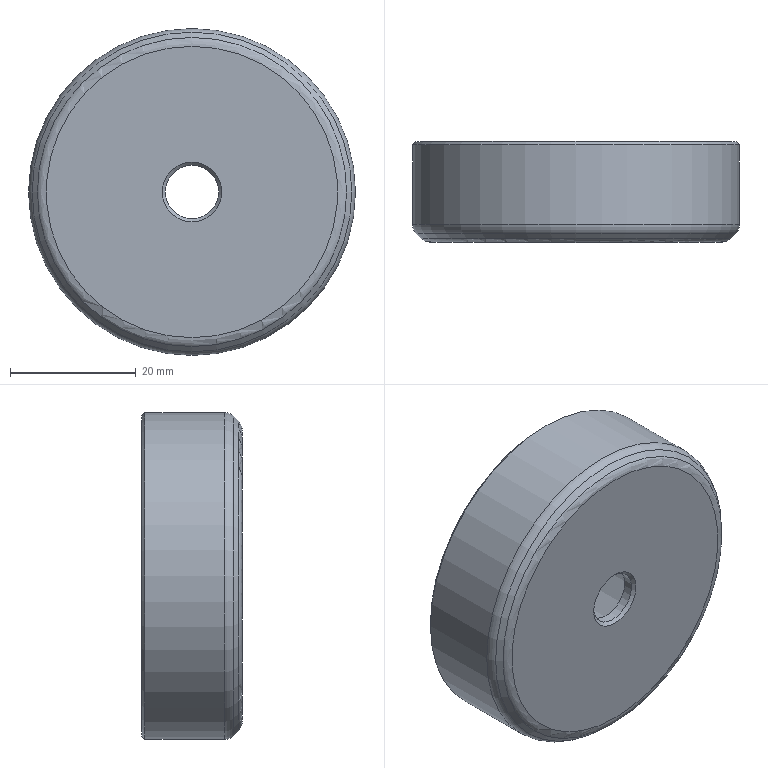Part | STEP file | PN_0026_default | 1 solid | 21 faces | box 52 x 16 x 52 mm | volume 11242 mm3 | torus 8 | cylinder 5 | plane 5 | cone 3 | commonest cylinder face diameters 8.5 x1 33 x1 37 x1 48 x1 52 x1
STEP:
#1=CARTESIAN_POINT('',(0.,0.,0.));
#2=DIRECTION('',(0.,0.,1.));
#3=DIRECTION('',(1.,0.,0.));
#4=AXIS2_PLACEMENT_3D('',#1,#2,#3);
#5=CARTESIAN_POINT('',(0.,0.5,4.25));
#6=VERTEX_POINT('',#5);
#7=CARTESIAN_POINT('',(0.,0.5,0.));
#8=DIRECTION('',(0.,-1.,0.));
#9=DIRECTION('',(0.,0.,1.));
#10=AXIS2_PLACEMENT_3D('',#7,#8,#9);
#11=CIRCLE('',#10,4.25);
#12=CARTESIAN_POINT('',(0.,49.95,0.));
#13=DIRECTION('',(0.,1.,0.));
#14=DIRECTION('',(0.,0.,1.));
#15=AXIS2_PLACEMENT_3D('',#12,#13,#14);
#16=CYLINDRICAL_SURFACE('',#15,4.25);
#17=CARTESIAN_POINT('',(6.283,-49.45));
#18=DIRECTION('',(-1.,0.));
#19=VECTOR('',#18,1.);
#20=LINE('',#17,#19);
#21=(GEOMETRIC_REPRESENTATION_CONTEXT(2)PARAMETRIC_REPRESENTATION_CONTEXT()REPRESENTATION_CONTEXT('',''));
#22=DEFINITIONAL_REPRESENTATION('',(#20),#21);
#23=PCURVE('',#16,#22);
#24=CARTESIAN_POINT('',(0.,0.,0.));
#25=DIRECTION('',(0.,-1.,0.));
#26=DIRECTION('',(0.,0.,-1.));
#27=AXIS2_PLACEMENT_3D('',#24,#25,#26);
#28=CONICAL_SURFACE('',#27,4.75,0.7854);
#29=CARTESIAN_POINT('',(3.142,-0.5));
#30=DIRECTION('',(1.,0.));
#31=VECTOR('',#30,1.);
#32=LINE('',#29,#31);
#33=(GEOMETRIC_REPRESENTATION_CONTEXT(2)PARAMETRIC_REPRESENTATION_CONTEXT()REPRESENTATION_CONTEXT('',''));
#34=DEFINITIONAL_REPRESENTATION('',(#32),#33);
#35=PCURVE('',#28,#34);
#36=SURFACE_CURVE('',#11,(#23,#35),.PCURVE_S1.);
#37=EDGE_CURVE('',#6,#6,#36,.T.);
#38=ORIENTED_EDGE('',*,*,#37,.F.);
#39=CARTESIAN_POINT('',(0.,2.,4.25));
#40=VERTEX_POINT('',#39);
#41=CARTESIAN_POINT('',(0.,0.5,4.25));
#42=CARTESIAN_POINT('',(0.,2.,4.25));
#43=B_SPLINE_CURVE_WITH_KNOTS('',1,(#41,#42),.UNSPECIFIED.,.F.,.F.,(2,2),(-49.45,-47.95),.PIECEWISE_BEZIER_KNOTS.);
#44=CARTESIAN_POINT('',(6.283,0.));
#45=DIRECTION('',(0.,1.));
#46=VECTOR('',#45,1.);
#47=LINE('',#44,#46);
#48=(GEOMETRIC_REPRESENTATION_CONTEXT(2)PARAMETRIC_REPRESENTATION_CONTEXT()REPRESENTATION_CONTEXT('',''));
#49=DEFINITIONAL_REPRESENTATION('',(#47),#48);
#50=PCURVE('',#16,#49);
#51=CARTESIAN_POINT('',(0.,0.));
#52=DIRECTION('',(0.,1.));
#53=VECTOR('',#52,1.);
#54=LINE('',#51,#53);
#55=(GEOMETRIC_REPRESENTATION_CONTEXT(2)PARAMETRIC_REPRESENTATION_CONTEXT()REPRESENTATION_CONTEXT('',''));
#56=DEFINITIONAL_REPRESENTATION('',(#54),#55);
#57=PCURVE('',#16,#56);
#58=SEAM_CURVE('',#43,(#50,#57),.PCURVE_S1.);
#59=EDGE_CURVE('',#6,#40,#58,.T.);
#60=ORIENTED_EDGE('',*,*,#59,.T.);
#61=CARTESIAN_POINT('',(0.,2.,0.));
#62=DIRECTION('',(0.,1.,0.));
#63=DIRECTION('',(0.,0.,1.));
#64=AXIS2_PLACEMENT_3D('',#61,#62,#63);
#65=CIRCLE('',#64,4.25);
#66=CARTESIAN_POINT('',(0.,-47.95));
#67=DIRECTION('',(1.,0.));
#68=VECTOR('',#67,1.);
#69=LINE('',#66,#68);
#70=(GEOMETRIC_REPRESENTATION_CONTEXT(2)PARAMETRIC_REPRESENTATION_CONTEXT()REPRESENTATION_CONTEXT('',''));
#71=DEFINITIONAL_REPRESENTATION('',(#69),#70);
#72=PCURVE('',#16,#71);
#73=CARTESIAN_POINT('',(16.,2.,0.));
#74=DIRECTION('',(0.,-1.,0.));
#75=DIRECTION('',(0.,0.,-1.));
#76=AXIS2_PLACEMENT_3D('',#73,#74,#75);
#77=PLANE('',#76);
#78=CARTESIAN_POINT('',(-4.25,-16.));
#79=CARTESIAN_POINT('',(-4.25,-8.639));
#80=CARTESIAN_POINT('',(2.125,-12.319));
#81=CARTESIAN_POINT('',(8.5,-16.));
#82=CARTESIAN_POINT('',(2.125,-19.681));
#83=CARTESIAN_POINT('',(-4.25,-23.361));
#84=CARTESIAN_POINT('',(-4.25,-16.));
#85=(BOUNDED_CURVE()B_SPLINE_CURVE(2,(#78,#79,#80,#81,#82,#83,#84),.UNSPECIFIED.,.T.,.F.)B_SPLINE_CURVE_WITH_KNOTS((1,2,2,2,2,1),(-2.094,0.,2.094,4.189,6.283,8.378),.UNSPECIFIED.)CURVE()GEOMETRIC_REPRESENTATION_ITEM()RATIONAL_B_SPLINE_CURVE((1.,0.5,1.,0.5,1.,0.5,1.))REPRESENTATION_ITEM(''));
#86=(GEOMETRIC_REPRESENTATION_CONTEXT(2)PARAMETRIC_REPRESENTATION_CONTEXT()REPRESENTATION_CONTEXT('',''));
#87=DEFINITIONAL_REPRESENTATION('',(#85),#86);
#88=PCURVE('',#77,#87);
#89=SURFACE_CURVE('',#65,(#72,#88),.PCURVE_S1.);
#90=EDGE_CURVE('',#40,#40,#89,.T.);
#91=ORIENTED_EDGE('',*,*,#90,.F.);
#92=ORIENTED_EDGE('',*,*,#59,.F.);
#93=EDGE_LOOP('',(#38,#60,#91,#92));
#94=FACE_BOUND('',#93,.F.);
#95=ADVANCED_FACE('',(#94),#16,.F.);
#96=CARTESIAN_POINT('',(0.,0.,4.75));
#97=VERTEX_POINT('',#96);
#98=CARTESIAN_POINT('',(0.,0.,0.));
#99=DIRECTION('',(0.,1.,0.));
#100=DIRECTION('',(0.,0.,1.));
#101=AXIS2_PLACEMENT_3D('',#98,#99,#100);
#102=CIRCLE('',#101,4.75);
#103=CARTESIAN_POINT('',(4.25,0.,0.));
#104=DIRECTION('',(0.,1.,0.));
#105=DIRECTION('',(0.,0.,1.));
#106=AXIS2_PLACEMENT_3D('',#103,#104,#105);
#107=PLANE('',#106);
#108=CARTESIAN_POINT('',(0.,-4.25));
#109=DIRECTION('',(1.,0.));
#110=AXIS2_PLACEMENT_2D('',#108,#109);
#111=CIRCLE('',#110,4.75);
#112=(GEOMETRIC_REPRESENTATION_CONTEXT(2)PARAMETRIC_REPRESENTATION_CONTEXT()REPRESENTATION_CONTEXT('',''));
#113=DEFINITIONAL_REPRESENTATION('',(#111),#112);
#114=PCURVE('',#107,#113);
#115=CARTESIAN_POINT('',(9.425,0.));
#116=DIRECTION('',(-1.,0.));
#117=VECTOR('',#116,1.);
#118=LINE('',#115,#117);
#119=(GEOMETRIC_REPRESENTATION_CONTEXT(2)PARAMETRIC_REPRESENTATION_CONTEXT()REPRESENTATION_CONTEXT('',''));
#120=DEFINITIONAL_REPRESENTATION('',(#118),#119);
#121=PCURVE('',#28,#120);
#122=SURFACE_CURVE('',#102,(#114,#121),.PCURVE_S1.);
#123=EDGE_CURVE('',#97,#97,#122,.T.);
#124=ORIENTED_EDGE('',*,*,#123,.T.);
#125=EDGE_LOOP('',(#124));
#126=FACE_BOUND('',#125,.T.);
#127=CARTESIAN_POINT('',(0.,0.,23.172));
#128=VERTEX_POINT('',#127);
#129=CARTESIAN_POINT('',(0.,0.,0.));
#130=DIRECTION('',(0.,-1.,0.));
#131=DIRECTION('',(0.,0.,1.));
#132=AXIS2_PLACEMENT_3D('',#129,#130,#131);
#133=CIRCLE('',#132,23.172);
#134=CARTESIAN_POINT('',(23.172,-4.25));
#135=CARTESIAN_POINT('',(23.172,-44.384));
#136=CARTESIAN_POINT('',(-11.586,-24.317));
#137=CARTESIAN_POINT('',(-46.343,-4.25));
#138=CARTESIAN_POINT('',(-11.586,15.817));
#139=CARTESIAN_POINT('',(23.172,35.884));
#140=CARTESIAN_POINT('',(23.172,-4.25));
#141=(BOUNDED_CURVE()B_SPLINE_CURVE(2,(#134,#135,#136,#137,#138,#139,#140),.UNSPECIFIED.,.T.,.F.)B_SPLINE_CURVE_WITH_KNOTS((1,2,2,2,2,1),(-2.094,0.,2.094,4.189,6.283,8.378),.UNSPECIFIED.)CURVE()GEOMETRIC_REPRESENTATION_ITEM()RATIONAL_B_SPLINE_CURVE((1.,0.5,1.,0.5,1.,0.5,1.))REPRESENTATION_ITEM(''));
#142=(GEOMETRIC_REPRESENTATION_CONTEXT(2)PARAMETRIC_REPRESENTATION_CONTEXT()REPRESENTATION_CONTEXT('',''));
#143=DEFINITIONAL_REPRESENTATION('',(#141),#142);
#144=PCURVE('',#107,#143);
#145=CARTESIAN_POINT('',(0.,2.,0.));
#146=DIRECTION('',(0.,1.,0.));
#147=DIRECTION('',(0.,0.,1.));
#148=AXIS2_PLACEMENT_3D('',#145,#146,#147);
#149=TOROIDAL_SURFACE('',#148,23.172,2.);
#150=CARTESIAN_POINT('',(6.283,4.712));
#151=DIRECTION('',(-1.,0.));
#152=VECTOR('',#151,1.);
#153=LINE('',#150,#152);
#154=(GEOMETRIC_REPRESENTATION_CONTEXT(2)PARAMETRIC_REPRESENTATION_CONTEXT()REPRESENTATION_CONTEXT('',''));
#155=DEFINITIONAL_REPRESENTATION('',(#153),#154);
#156=PCURVE('',#149,#155);
#157=SURFACE_CURVE('',#133,(#144,#156),.PCURVE_S1.);
#158=EDGE_CURVE('',#128,#128,#157,.T.);
#159=ORIENTED_EDGE('',*,*,#158,.T.);
#160=EDGE_LOOP('',(#159));
#161=FACE_BOUND('',#160,.T.);
#162=ADVANCED_FACE('',(#126,#161),#107,.F.);
#163=CARTESIAN_POINT('',(0.,1.414,-25.414));
#164=VERTEX_POINT('',#163);
#165=CARTESIAN_POINT('',(0.,1.414,0.));
#166=DIRECTION('',(0.,-1.,0.));
#167=DIRECTION('',(0.,0.,-1.));
#168=AXIS2_PLACEMENT_3D('',#165,#166,#167);
#169=CIRCLE('',#168,25.414);
#170=CARTESIAN_POINT('',(0.,0.,0.));
#171=DIRECTION('',(0.,1.,0.));
#172=DIRECTION('',(0.,0.,1.));
#173=AXIS2_PLACEMENT_3D('',#170,#171,#172);
#174=CONICAL_SURFACE('',#173,24.,0.7854);
#175=CARTESIAN_POINT('',(9.425,1.414));
#176=DIRECTION('',(-1.,0.));
#177=VECTOR('',#176,1.);
#178=LINE('',#175,#177);
#179=(GEOMETRIC_REPRESENTATION_CONTEXT(2)PARAMETRIC_REPRESENTATION_CONTEXT()REPRESENTATION_CONTEXT('',''));
#180=DEFINITIONAL_REPRESENTATION('',(#178),#179);
#181=PCURVE('',#174,#180);
#182=CARTESIAN_POINT('',(0.,2.828,0.));
#183=DIRECTION('',(0.,-1.,0.));
#184=DIRECTION('',(0.,0.,-1.));
#185=AXIS2_PLACEMENT_3D('',#182,#183,#184);
#186=TOROIDAL_SURFACE('',#185,24.,2.);
#187=CARTESIAN_POINT('',(0.,7.069));
#188=DIRECTION('',(1.,0.));
#189=VECTOR('',#188,1.);
#190=LINE('',#187,#189);
#191=(GEOMETRIC_REPRESENTATION_CONTEXT(2)PARAMETRIC_REPRESENTATION_CONTEXT()REPRESENTATION_CONTEXT('',''));
#192=DEFINITIONAL_REPRESENTATION('',(#190),#191);
#193=PCURVE('',#186,#192);
#194=SURFACE_CURVE('',#169,(#181,#193),.PCURVE_S1.);
#195=EDGE_CURVE('',#164,#164,#194,.T.);
#196=ORIENTED_EDGE('',*,*,#195,.T.);
#197=CARTESIAN_POINT('',(0.,0.5858,-24.586));
#198=VERTEX_POINT('',#197);
#199=CARTESIAN_POINT('',(0.,0.5858,-24.586));
#200=CARTESIAN_POINT('',(0.,1.414,-25.414));
#201=B_SPLINE_CURVE_WITH_KNOTS('',1,(#199,#200),.UNSPECIFIED.,.F.,.F.,(2,2),(0.8284,2.),.PIECEWISE_BEZIER_KNOTS.);
#202=CARTESIAN_POINT('',(3.142,0.));
#203=DIRECTION('',(0.,1.));
#204=VECTOR('',#203,1.);
#205=LINE('',#202,#204);
#206=(GEOMETRIC_REPRESENTATION_CONTEXT(2)PARAMETRIC_REPRESENTATION_CONTEXT()REPRESENTATION_CONTEXT('',''));
#207=DEFINITIONAL_REPRESENTATION('',(#205),#206);
#208=PCURVE('',#174,#207);
#209=CARTESIAN_POINT('',(9.425,0.));
#210=DIRECTION('',(0.,1.));
#211=VECTOR('',#210,1.);
#212=LINE('',#209,#211);
#213=(GEOMETRIC_REPRESENTATION_CONTEXT(2)PARAMETRIC_REPRESENTATION_CONTEXT()REPRESENTATION_CONTEXT('',''));
#214=DEFINITIONAL_REPRESENTATION('',(#212),#213);
#215=PCURVE('',#174,#214);
#216=SEAM_CURVE('',#201,(#208,#215),.PCURVE_S1.);
#217=EDGE_CURVE('',#198,#164,#216,.T.);
#218=ORIENTED_EDGE('',*,*,#217,.F.);
#219=CARTESIAN_POINT('',(0.,0.5858,24.586));
#220=VERTEX_POINT('',#219);
#221=CARTESIAN_POINT('',(0.,0.5858,0.));
#222=DIRECTION('',(0.,1.,0.));
#223=DIRECTION('',(0.,0.,-1.));
#224=AXIS2_PLACEMENT_3D('',#221,#222,#223);
#225=CIRCLE('',#224,24.586);
#226=CARTESIAN_POINT('',(3.142,0.5858));
#227=DIRECTION('',(1.,0.));
#228=VECTOR('',#227,1.);
#229=LINE('',#226,#228);
#230=(GEOMETRIC_REPRESENTATION_CONTEXT(2)PARAMETRIC_REPRESENTATION_CONTEXT()REPRESENTATION_CONTEXT('',''));
#231=DEFINITIONAL_REPRESENTATION('',(#229),#230);
#232=PCURVE('',#174,#231);
#233=CARTESIAN_POINT('',(3.142,5.498));
#234=DIRECTION('',(1.,0.));
#235=VECTOR('',#234,1.);
#236=LINE('',#233,#235);
#237=(GEOMETRIC_REPRESENTATION_CONTEXT(2)PARAMETRIC_REPRESENTATION_CONTEXT()REPRESENTATION_CONTEXT('',''));
#238=DEFINITIONAL_REPRESENTATION('',(#236),#237);
#239=PCURVE('',#149,#238);
#240=SURFACE_CURVE('',#225,(#232,#239),.PCURVE_S1.);
#241=EDGE_CURVE('',#198,#220,#240,.T.);
#242=ORIENTED_EDGE('',*,*,#241,.T.);
#243=CARTESIAN_POINT('',(0.,0.5858,0.));
#244=DIRECTION('',(0.,1.,0.));
#245=DIRECTION('',(0.,0.,-1.));
#246=AXIS2_PLACEMENT_3D('',#243,#244,#245);
#247=CIRCLE('',#246,24.586);
#248=CARTESIAN_POINT('',(3.142,0.5858));
#249=DIRECTION('',(1.,0.));
#250=VECTOR('',#249,1.);
#251=LINE('',#248,#250);
#252=(GEOMETRIC_REPRESENTATION_CONTEXT(2)PARAMETRIC_REPRESENTATION_CONTEXT()REPRESENTATION_CONTEXT('',''));
#253=DEFINITIONAL_REPRESENTATION('',(#251),#252);
#254=PCURVE('',#174,#253);
#255=CARTESIAN_POINT('',(-3.142,5.498));
#256=DIRECTION('',(1.,0.));
#257=VECTOR('',#256,1.);
#258=LINE('',#255,#257);
#259=(GEOMETRIC_REPRESENTATION_CONTEXT(2)PARAMETRIC_REPRESENTATION_CONTEXT()REPRESENTATION_CONTEXT('',''));
#260=DEFINITIONAL_REPRESENTATION('',(#258),#259);
#261=PCURVE('',#149,#260);
#262=SURFACE_CURVE('',#247,(#254,#261),.PCURVE_S1.);
#263=EDGE_CURVE('',#220,#198,#262,.T.);
#264=ORIENTED_EDGE('',*,*,#263,.T.);
#265=ORIENTED_EDGE('',*,*,#217,.T.);
#266=EDGE_LOOP('',(#196,#218,#242,#264,#265));
#267=FACE_BOUND('',#266,.T.);
#268=ADVANCED_FACE('',(#267),#174,.T.);
#269=CARTESIAN_POINT('',(0.,2.828,-26.));
#270=VERTEX_POINT('',#269);
#271=CARTESIAN_POINT('',(0.,2.828,26.));
#272=VERTEX_POINT('',#271);
#273=CARTESIAN_POINT('',(0.,2.828,0.));
#274=DIRECTION('',(0.,1.,0.));
#275=DIRECTION('',(0.,0.,-1.));
#276=AXIS2_PLACEMENT_3D('',#273,#274,#275);
#277=CIRCLE('',#276,26.);
#278=CARTESIAN_POINT('',(0.,49.95,0.));
#279=DIRECTION('',(0.,1.,0.));
#280=DIRECTION('',(0.,0.,1.));
#281=AXIS2_PLACEMENT_3D('',#278,#279,#280);
#282=CYLINDRICAL_SURFACE('',#281,26.);
#283=CARTESIAN_POINT('',(3.142,-47.121));
#284=DIRECTION('',(1.,0.));
#285=VECTOR('',#284,1.);
#286=LINE('',#283,#285);
#287=(GEOMETRIC_REPRESENTATION_CONTEXT(2)PARAMETRIC_REPRESENTATION_CONTEXT()REPRESENTATION_CONTEXT('',''));
#288=DEFINITIONAL_REPRESENTATION('',(#286),#287);
#289=PCURVE('',#282,#288);
#290=CARTESIAN_POINT('',(6.283,6.283));
#291=DIRECTION('',(-1.,0.));
#292=VECTOR('',#291,1.);
#293=LINE('',#290,#292);
#294=(GEOMETRIC_REPRESENTATION_CONTEXT(2)PARAMETRIC_REPRESENTATION_CONTEXT()REPRESENTATION_CONTEXT('',''));
#295=DEFINITIONAL_REPRESENTATION('',(#293),#294);
#296=PCURVE('',#186,#295);
#297=SURFACE_CURVE('',#277,(#289,#296),.PCURVE_S1.);
#298=EDGE_CURVE('',#270,#272,#297,.T.);
#299=ORIENTED_EDGE('',*,*,#298,.T.);
#300=CARTESIAN_POINT('',(0.,15.5,26.));
#301=VERTEX_POINT('',#300);
#302=CARTESIAN_POINT('',(0.,2.828,26.));
#303=CARTESIAN_POINT('',(0.,15.5,26.));
#304=B_SPLINE_CURVE_WITH_KNOTS('',1,(#302,#303),.UNSPECIFIED.,.F.,.F.,(2,2),(-47.121,-34.45),.PIECEWISE_BEZIER_KNOTS.);
#305=CARTESIAN_POINT('',(6.283,0.));
#306=DIRECTION('',(0.,1.));
#307=VECTOR('',#306,1.);
#308=LINE('',#305,#307);
#309=(GEOMETRIC_REPRESENTATION_CONTEXT(2)PARAMETRIC_REPRESENTATION_CONTEXT()REPRESENTATION_CONTEXT('',''));
#310=DEFINITIONAL_REPRESENTATION('',(#308),#309);
#311=PCURVE('',#282,#310);
#312=CARTESIAN_POINT('',(0.,0.));
#313=DIRECTION('',(0.,1.));
#314=VECTOR('',#313,1.);
#315=LINE('',#312,#314);
#316=(GEOMETRIC_REPRESENTATION_CONTEXT(2)PARAMETRIC_REPRESENTATION_CONTEXT()REPRESENTATION_CONTEXT('',''));
#317=DEFINITIONAL_REPRESENTATION('',(#315),#316);
#318=PCURVE('',#282,#317);
#319=SEAM_CURVE('',#304,(#311,#318),.PCURVE_S1.);
#320=EDGE_CURVE('',#272,#301,#319,.T.);
#321=ORIENTED_EDGE('',*,*,#320,.T.);
#322=CARTESIAN_POINT('',(0.,15.5,0.));
#323=DIRECTION('',(0.,1.,0.));
#324=DIRECTION('',(0.,0.,1.));
#325=AXIS2_PLACEMENT_3D('',#322,#323,#324);
#326=CIRCLE('',#325,26.);
#327=CARTESIAN_POINT('',(0.,-34.45));
#328=DIRECTION('',(1.,0.));
#329=VECTOR('',#328,1.);
#330=LINE('',#327,#329);
#331=(GEOMETRIC_REPRESENTATION_CONTEXT(2)PARAMETRIC_REPRESENTATION_CONTEXT()REPRESENTATION_CONTEXT('',''));
#332=DEFINITIONAL_REPRESENTATION('',(#330),#331);
#333=PCURVE('',#282,#332);
#334=CARTESIAN_POINT('',(0.,15.5,0.));
#335=DIRECTION('',(0.,-1.,0.));
#336=DIRECTION('',(0.,0.,-1.));
#337=AXIS2_PLACEMENT_3D('',#334,#335,#336);
#338=CONICAL_SURFACE('',#337,26.,0.7854);
#339=CARTESIAN_POINT('',(9.425,0.));
#340=DIRECTION('',(-1.,0.));
#341=VECTOR('',#340,1.);
#342=LINE('',#339,#341);
#343=(GEOMETRIC_REPRESENTATION_CONTEXT(2)PARAMETRIC_REPRESENTATION_CONTEXT()REPRESENTATION_CONTEXT('',''));
#344=DEFINITIONAL_REPRESENTATION('',(#342),#343);
#345=PCURVE('',#338,#344);
#346=SURFACE_CURVE('',#326,(#333,#345),.PCURVE_S1.);
#347=EDGE_CURVE('',#301,#301,#346,.T.);
#348=ORIENTED_EDGE('',*,*,#347,.F.);
#349=ORIENTED_EDGE('',*,*,#320,.F.);
#350=CARTESIAN_POINT('',(0.,2.828,0.));
#351=DIRECTION('',(0.,1.,0.));
#352=DIRECTION('',(0.,0.,-1.));
#353=AXIS2_PLACEMENT_3D('',#350,#351,#352);
#354=CIRCLE('',#353,26.);
#355=CARTESIAN_POINT('',(-3.142,-47.121));
#356=DIRECTION('',(1.,0.));
#357=VECTOR('',#356,1.);
#358=LINE('',#355,#357);
#359=(GEOMETRIC_REPRESENTATION_CONTEXT(2)PARAMETRIC_REPRESENTATION_CONTEXT()REPRESENTATION_CONTEXT('',''));
#360=DEFINITIONAL_REPRESENTATION('',(#358),#359);
#361=PCURVE('',#282,#360);
#362=CARTESIAN_POINT('',(6.283,6.283));
#363=DIRECTION('',(-1.,0.));
#364=VECTOR('',#363,1.);
#365=LINE('',#362,#364);
#366=(GEOMETRIC_REPRESENTATION_CONTEXT(2)PARAMETRIC_REPRESENTATION_CONTEXT()REPRESENTATION_CONTEXT('',''));
#367=DEFINITIONAL_REPRESENTATION('',(#365),#366);
#368=PCURVE('',#186,#367);
#369=SURFACE_CURVE('',#354,(#361,#368),.PCURVE_S1.);
#370=EDGE_CURVE('',#272,#270,#369,.T.);
#371=ORIENTED_EDGE('',*,*,#370,.T.);
#372=EDGE_LOOP('',(#299,#321,#348,#349,#371));
#373=FACE_BOUND('',#372,.T.);
#374=ADVANCED_FACE('',(#373),#282,.T.);
#375=CARTESIAN_POINT('',(0.,16.,25.5));
#376=VERTEX_POINT('',#375);
#377=CARTESIAN_POINT('',(0.,16.,0.));
#378=DIRECTION('',(0.,1.,0.));
#379=DIRECTION('',(0.,0.,1.));
#380=AXIS2_PLACEMENT_3D('',#377,#378,#379);
#381=CIRCLE('',#380,25.5);
#382=CARTESIAN_POINT('',(9.425,-0.5));
#383=DIRECTION('',(-1.,0.));
#384=VECTOR('',#383,1.);
#385=LINE('',#382,#384);
#386=(GEOMETRIC_REPRESENTATION_CONTEXT(2)PARAMETRIC_REPRESENTATION_CONTEXT()REPRESENTATION_CONTEXT('',''));
#387=DEFINITIONAL_REPRESENTATION('',(#385),#386);
#388=PCURVE('',#338,#387);
#389=CARTESIAN_POINT('',(25.5,16.,0.));
#390=DIRECTION('',(0.,-1.,0.));
#391=DIRECTION('',(0.,0.,-1.));
#392=AXIS2_PLACEMENT_3D('',#389,#390,#391);
#393=PLANE('',#392);
#394=CARTESIAN_POINT('',(-25.5,-25.5));
#395=CARTESIAN_POINT('',(-25.5,18.667));
#396=CARTESIAN_POINT('',(12.75,-3.416));
#397=CARTESIAN_POINT('',(51.,-25.5));
#398=CARTESIAN_POINT('',(12.75,-47.584));
#399=CARTESIAN_POINT('',(-25.5,-69.667));
#400=CARTESIAN_POINT('',(-25.5,-25.5));
#401=(BOUNDED_CURVE()B_SPLINE_CURVE(2,(#394,#395,#396,#397,#398,#399,#400),.UNSPECIFIED.,.T.,.F.)B_SPLINE_CURVE_WITH_KNOTS((1,2,2,2,2,1),(-2.094,0.,2.094,4.189,6.283,8.378),.UNSPECIFIED.)CURVE()GEOMETRIC_REPRESENTATION_ITEM()RATIONAL_B_SPLINE_CURVE((1.,0.5,1.,0.5,1.,0.5,1.))REPRESENTATION_ITEM(''));
#402=(GEOMETRIC_REPRESENTATION_CONTEXT(2)PARAMETRIC_REPRESENTATION_CONTEXT()REPRESENTATION_CONTEXT('',''));
#403=DEFINITIONAL_REPRESENTATION('',(#401),#402);
#404=PCURVE('',#393,#403);
#405=SURFACE_CURVE('',#381,(#388,#404),.PCURVE_S1.);
#406=EDGE_CURVE('',#376,#376,#405,.T.);
#407=ORIENTED_EDGE('',*,*,#406,.F.);
#408=CARTESIAN_POINT('',(0.,16.,25.5));
#409=CARTESIAN_POINT('',(0.,15.5,26.));
#410=B_SPLINE_CURVE_WITH_KNOTS('',1,(#408,#409),.UNSPECIFIED.,.F.,.F.,(2,2),(-0.7071,0.),.PIECEWISE_BEZIER_KNOTS.);
#411=CARTESIAN_POINT('',(9.425,0.));
#412=DIRECTION('',(0.,1.));
#413=VECTOR('',#412,1.);
#414=LINE('',#411,#413);
#415=(GEOMETRIC_REPRESENTATION_CONTEXT(2)PARAMETRIC_REPRESENTATION_CONTEXT()REPRESENTATION_CONTEXT('',''));
#416=DEFINITIONAL_REPRESENTATION('',(#414),#415);
#417=PCURVE('',#338,#416);
#418=CARTESIAN_POINT('',(3.142,0.));
#419=DIRECTION('',(0.,1.));
#420=VECTOR('',#419,1.);
#421=LINE('',#418,#420);
#422=(GEOMETRIC_REPRESENTATION_CONTEXT(2)PARAMETRIC_REPRESENTATION_CONTEXT()REPRESENTATION_CONTEXT('',''));
#423=DEFINITIONAL_REPRESENTATION('',(#421),#422);
#424=PCURVE('',#338,#423);
#425=SEAM_CURVE('',#410,(#417,#424),.PCURVE_S1.);
#426=EDGE_CURVE('',#376,#301,#425,.T.);
#427=ORIENTED_EDGE('',*,*,#426,.T.);
#428=ORIENTED_EDGE('',*,*,#347,.T.);
#429=ORIENTED_EDGE('',*,*,#426,.F.);
#430=EDGE_LOOP('',(#407,#427,#428,#429));
#431=FACE_BOUND('',#430,.T.);
#432=ADVANCED_FACE('',(#431),#338,.T.);
#433=CARTESIAN_POINT('',(0.,16.,24.5));
#434=VERTEX_POINT('',#433);
#435=CARTESIAN_POINT('',(0.,16.,0.));
#436=DIRECTION('',(0.,1.,0.));
#437=DIRECTION('',(0.,0.,1.));
#438=AXIS2_PLACEMENT_3D('',#435,#436,#437);
#439=CIRCLE('',#438,24.5);
#440=CARTESIAN_POINT('',(-24.5,-25.5));
#441=CARTESIAN_POINT('',(-24.5,16.935));
#442=CARTESIAN_POINT('',(12.25,-4.282));
#443=CARTESIAN_POINT('',(49.,-25.5));
#444=CARTESIAN_POINT('',(12.25,-46.718));
#445=CARTESIAN_POINT('',(-24.5,-67.935));
#446=CARTESIAN_POINT('',(-24.5,-25.5));
#447=(BOUNDED_CURVE()B_SPLINE_CURVE(2,(#440,#441,#442,#443,#444,#445,#446),.UNSPECIFIED.,.T.,.F.)B_SPLINE_CURVE_WITH_KNOTS((1,2,2,2,2,1),(-2.094,0.,2.094,4.189,6.283,8.378),.UNSPECIFIED.)CURVE()GEOMETRIC_REPRESENTATION_ITEM()RATIONAL_B_SPLINE_CURVE((1.,0.5,1.,0.5,1.,0.5,1.))REPRESENTATION_ITEM(''));
#448=(GEOMETRIC_REPRESENTATION_CONTEXT(2)PARAMETRIC_REPRESENTATION_CONTEXT()REPRESENTATION_CONTEXT('',''));
#449=DEFINITIONAL_REPRESENTATION('',(#447),#448);
#450=PCURVE('',#393,#449);
#451=CARTESIAN_POINT('',(0.,15.5,0.));
#452=DIRECTION('',(0.,1.,0.));
#453=DIRECTION('',(0.,0.,1.));
#454=AXIS2_PLACEMENT_3D('',#451,#452,#453);
#455=TOROIDAL_SURFACE('',#454,24.5,0.5);
#456=CARTESIAN_POINT('',(0.,7.854));
#457=DIRECTION('',(1.,0.));
#458=VECTOR('',#457,1.);
#459=LINE('',#456,#458);
#460=(GEOMETRIC_REPRESENTATION_CONTEXT(2)PARAMETRIC_REPRESENTATION_CONTEXT()REPRESENTATION_CONTEXT('',''));
#461=DEFINITIONAL_REPRESENTATION('',(#459),#460);
#462=PCURVE('',#455,#461);
#463=SURFACE_CURVE('',#439,(#450,#462),.PCURVE_S1.);
#464=EDGE_CURVE('',#434,#434,#463,.T.);
#465=ORIENTED_EDGE('',*,*,#464,.F.);
#466=EDGE_LOOP('',(#465));
#467=FACE_BOUND('',#466,.T.);
#468=ORIENTED_EDGE('',*,*,#406,.T.);
#469=EDGE_LOOP('',(#468));
#470=FACE_BOUND('',#469,.T.);
#471=ADVANCED_FACE('',(#467,#470),#393,.F.);
#472=CARTESIAN_POINT('',(0.,15.5,24.));
#473=VERTEX_POINT('',#472);
#474=CARTESIAN_POINT('',(0.,15.5,0.));
#475=DIRECTION('',(0.,1.,0.));
#476=DIRECTION('',(0.,0.,1.));
#477=AXIS2_PLACEMENT_3D('',#474,#475,#476);
#478=CIRCLE('',#477,24.);
#479=CARTESIAN_POINT('',(0.,9.425));
#480=DIRECTION('',(1.,0.));
#481=VECTOR('',#480,1.);
#482=LINE('',#479,#481);
#483=(GEOMETRIC_REPRESENTATION_CONTEXT(2)PARAMETRIC_REPRESENTATION_CONTEXT()REPRESENTATION_CONTEXT('',''));
#484=DEFINITIONAL_REPRESENTATION('',(#482),#483);
#485=PCURVE('',#455,#484);
#486=CARTESIAN_POINT('',(0.,49.95,0.));
#487=DIRECTION('',(0.,1.,0.));
#488=DIRECTION('',(0.,0.,1.));
#489=AXIS2_PLACEMENT_3D('',#486,#487,#488);
#490=CYLINDRICAL_SURFACE('',#489,24.);
#491=CARTESIAN_POINT('',(0.,-34.45));
#492=DIRECTION('',(1.,0.));
#493=VECTOR('',#492,1.);
#494=LINE('',#491,#493);
#495=(GEOMETRIC_REPRESENTATION_CONTEXT(2)PARAMETRIC_REPRESENTATION_CONTEXT()REPRESENTATION_CONTEXT('',''));
#496=DEFINITIONAL_REPRESENTATION('',(#494),#495);
#497=PCURVE('',#490,#496);
#498=SURFACE_CURVE('',#478,(#485,#497),.PCURVE_S1.);
#499=EDGE_CURVE('',#473,#473,#498,.T.);
#500=ORIENTED_EDGE('',*,*,#499,.F.);
#501=CARTESIAN_POINT('',(0.,16.,24.5));
#502=CARTESIAN_POINT('',(0.,16.,24.366));
#503=CARTESIAN_POINT('',(0.,15.957,24.236));
#504=CARTESIAN_POINT('',(0.,15.876,24.124));
#505=CARTESIAN_POINT('',(0.,15.764,24.043));
#506=CARTESIAN_POINT('',(0.,15.634,24.));
#507=CARTESIAN_POINT('',(0.,15.5,24.));
#508=(BOUNDED_CURVE()B_SPLINE_CURVE(6,(#501,#502,#503,#504,#505,#506,#507),.UNSPECIFIED.,.F.,.F.)B_SPLINE_CURVE_WITH_KNOTS((7,7),(1.571,3.142),.PIECEWISE_BEZIER_KNOTS.)CURVE()GEOMETRIC_REPRESENTATION_ITEM()RATIONAL_B_SPLINE_CURVE((1.031,1.01,0.9979,0.994,0.9979,1.01,1.031))REPRESENTATION_ITEM(''));
#509=CARTESIAN_POINT('',(0.,6.283));
#510=DIRECTION('',(0.,1.));
#511=VECTOR('',#510,1.);
#512=LINE('',#509,#511);
#513=(GEOMETRIC_REPRESENTATION_CONTEXT(2)PARAMETRIC_REPRESENTATION_CONTEXT()REPRESENTATION_CONTEXT('',''));
#514=DEFINITIONAL_REPRESENTATION('',(#512),#513);
#515=PCURVE('',#455,#514);
#516=CARTESIAN_POINT('',(6.283,6.283));
#517=DIRECTION('',(0.,1.));
#518=VECTOR('',#517,1.);
#519=LINE('',#516,#518);
#520=(GEOMETRIC_REPRESENTATION_CONTEXT(2)PARAMETRIC_REPRESENTATION_CONTEXT()REPRESENTATION_CONTEXT('',''));
#521=DEFINITIONAL_REPRESENTATION('',(#519),#520);
#522=PCURVE('',#455,#521);
#523=SEAM_CURVE('',#508,(#515,#522),.PCURVE_S1.);
#524=EDGE_CURVE('',#434,#473,#523,.T.);
#525=ORIENTED_EDGE('',*,*,#524,.F.);
#526=ORIENTED_EDGE('',*,*,#464,.T.);
#527=ORIENTED_EDGE('',*,*,#524,.T.);
#528=EDGE_LOOP('',(#500,#525,#526,#527));
#529=FACE_BOUND('',#528,.T.);
#530=ADVANCED_FACE('',(#529),#455,.T.);
#531=CARTESIAN_POINT('',(0.,2.5,24.));
#532=VERTEX_POINT('',#531);
#533=CARTESIAN_POINT('',(0.,2.5,0.));
#534=DIRECTION('',(0.,1.,0.));
#535=DIRECTION('',(0.,0.,1.));
#536=AXIS2_PLACEMENT_3D('',#533,#534,#535);
#537=CIRCLE('',#536,24.);
#538=CARTESIAN_POINT('',(0.,-47.45));
#539=DIRECTION('',(1.,0.));
#540=VECTOR('',#539,1.);
#541=LINE('',#538,#540);
#542=(GEOMETRIC_REPRESENTATION_CONTEXT(2)PARAMETRIC_REPRESENTATION_CONTEXT()REPRESENTATION_CONTEXT('',''));
#543=DEFINITIONAL_REPRESENTATION('',(#541),#542);
#544=PCURVE('',#490,#543);
#545=CARTESIAN_POINT('',(0.,2.5,0.));
#546=DIRECTION('',(0.,1.,0.));
#547=DIRECTION('',(0.,0.,1.));
#548=AXIS2_PLACEMENT_3D('',#545,#546,#547);
#549=TOROIDAL_SURFACE('',#548,23.5,0.5);
#550=CARTESIAN_POINT('',(0.,6.283));
#551=DIRECTION('',(1.,0.));
#552=VECTOR('',#551,1.);
#553=LINE('',#550,#552);
#554=(GEOMETRIC_REPRESENTATION_CONTEXT(2)PARAMETRIC_REPRESENTATION_CONTEXT()REPRESENTATION_CONTEXT('',''));
#555=DEFINITIONAL_REPRESENTATION('',(#553),#554);
#556=PCURVE('',#549,#555);
#557=SURFACE_CURVE('',#537,(#544,#556),.PCURVE_S1.);
#558=EDGE_CURVE('',#532,#532,#557,.T.);
#559=ORIENTED_EDGE('',*,*,#558,.T.);
#560=CARTESIAN_POINT('',(0.,2.5,24.));
#561=CARTESIAN_POINT('',(0.,15.5,24.));
#562=B_SPLINE_CURVE_WITH_KNOTS('',1,(#560,#561),.UNSPECIFIED.,.F.,.F.,(2,2),(-47.45,-34.45),.PIECEWISE_BEZIER_KNOTS.);
#563=CARTESIAN_POINT('',(6.283,0.));
#564=DIRECTION('',(0.,1.));
#565=VECTOR('',#564,1.);
#566=LINE('',#563,#565);
#567=(GEOMETRIC_REPRESENTATION_CONTEXT(2)PARAMETRIC_REPRESENTATION_CONTEXT()REPRESENTATION_CONTEXT('',''));
#568=DEFINITIONAL_REPRESENTATION('',(#566),#567);
#569=PCURVE('',#490,#568);
#570=CARTESIAN_POINT('',(0.,0.));
#571=DIRECTION('',(0.,1.));
#572=VECTOR('',#571,1.);
#573=LINE('',#570,#572);
#574=(GEOMETRIC_REPRESENTATION_CONTEXT(2)PARAMETRIC_REPRESENTATION_CONTEXT()REPRESENTATION_CONTEXT('',''));
#575=DEFINITIONAL_REPRESENTATION('',(#573),#574);
#576=PCURVE('',#490,#575);
#577=SEAM_CURVE('',#562,(#569,#576),.PCURVE_S1.);
#578=EDGE_CURVE('',#532,#473,#577,.T.);
#579=ORIENTED_EDGE('',*,*,#578,.T.);
#580=ORIENTED_EDGE('',*,*,#499,.F.);
#581=ORIENTED_EDGE('',*,*,#578,.F.);
#582=EDGE_LOOP('',(#559,#579,#580,#581));
#583=FACE_BOUND('',#582,.F.);
#584=ADVANCED_FACE('',(#583),#490,.F.);
#585=CARTESIAN_POINT('',(0.,2.,23.5));
#586=VERTEX_POINT('',#585);
#587=CARTESIAN_POINT('',(0.,2.,0.));
#588=DIRECTION('',(0.,1.,0.));
#589=DIRECTION('',(0.,0.,1.));
#590=AXIS2_PLACEMENT_3D('',#587,#588,#589);
#591=CIRCLE('',#590,23.5);
#592=CARTESIAN_POINT('',(0.,4.712));
#593=DIRECTION('',(1.,0.));
#594=VECTOR('',#593,1.);
#595=LINE('',#592,#594);
#596=(GEOMETRIC_REPRESENTATION_CONTEXT(2)PARAMETRIC_REPRESENTATION_CONTEXT()REPRESENTATION_CONTEXT('',''));
#597=DEFINITIONAL_REPRESENTATION('',(#595),#596);
#598=PCURVE('',#549,#597);
#599=CARTESIAN_POINT('',(23.5,2.,0.));
#600=DIRECTION('',(0.,-1.,0.));
#601=DIRECTION('',(0.,0.,-1.));
#602=AXIS2_PLACEMENT_3D('',#599,#600,#601);
#603=PLANE('',#602);
#604=CARTESIAN_POINT('',(-23.5,-23.5));
#605=CARTESIAN_POINT('',(-23.5,17.203));
#606=CARTESIAN_POINT('',(11.75,-3.148));
#607=CARTESIAN_POINT('',(47.,-23.5));
#608=CARTESIAN_POINT('',(11.75,-43.852));
#609=CARTESIAN_POINT('',(-23.5,-64.203));
#610=CARTESIAN_POINT('',(-23.5,-23.5));
#611=(BOUNDED_CURVE()B_SPLINE_CURVE(2,(#604,#605,#606,#607,#608,#609,#610),.UNSPECIFIED.,.T.,.F.)B_SPLINE_CURVE_WITH_KNOTS((1,2,2,2,2,1),(-2.094,0.,2.094,4.189,6.283,8.378),.UNSPECIFIED.)CURVE()GEOMETRIC_REPRESENTATION_ITEM()RATIONAL_B_SPLINE_CURVE((1.,0.5,1.,0.5,1.,0.5,1.))REPRESENTATION_ITEM(''));
#612=(GEOMETRIC_REPRESENTATION_CONTEXT(2)PARAMETRIC_REPRESENTATION_CONTEXT()REPRESENTATION_CONTEXT('',''));
#613=DEFINITIONAL_REPRESENTATION('',(#611),#612);
#614=PCURVE('',#603,#613);
#615=SURFACE_CURVE('',#591,(#598,#614),.PCURVE_S1.);
#616=EDGE_CURVE('',#586,#586,#615,.T.);
#617=ORIENTED_EDGE('',*,*,#616,.T.);
#618=CARTESIAN_POINT('',(0.,2.,23.5));
#619=CARTESIAN_POINT('',(0.,2.,23.634));
#620=CARTESIAN_POINT('',(0.,2.043,23.764));
#621=CARTESIAN_POINT('',(0.,2.124,23.876));
#622=CARTESIAN_POINT('',(0.,2.236,23.957));
#623=CARTESIAN_POINT('',(0.,2.366,24.));
#624=CARTESIAN_POINT('',(0.,2.5,24.));
#625=(BOUNDED_CURVE()B_SPLINE_CURVE(6,(#618,#619,#620,#621,#622,#623,#624),.UNSPECIFIED.,.F.,.F.)B_SPLINE_CURVE_WITH_KNOTS((7,7),(4.712,6.283),.PIECEWISE_BEZIER_KNOTS.)CURVE()GEOMETRIC_REPRESENTATION_ITEM()RATIONAL_B_SPLINE_CURVE((1.031,1.01,0.9979,0.994,0.9979,1.01,1.031))REPRESENTATION_ITEM(''));
#626=CARTESIAN_POINT('',(6.283,0.));
#627=DIRECTION('',(0.,1.));
#628=VECTOR('',#627,1.);
#629=LINE('',#626,#628);
#630=(GEOMETRIC_REPRESENTATION_CONTEXT(2)PARAMETRIC_REPRESENTATION_CONTEXT()REPRESENTATION_CONTEXT('',''));
#631=DEFINITIONAL_REPRESENTATION('',(#629),#630);
#632=PCURVE('',#549,#631);
#633=CARTESIAN_POINT('',(0.,0.));
#634=DIRECTION('',(0.,1.));
#635=VECTOR('',#634,1.);
#636=LINE('',#633,#635);
#637=(GEOMETRIC_REPRESENTATION_CONTEXT(2)PARAMETRIC_REPRESENTATION_CONTEXT()REPRESENTATION_CONTEXT('',''));
#638=DEFINITIONAL_REPRESENTATION('',(#636),#637);
#639=PCURVE('',#549,#638);
#640=SEAM_CURVE('',#625,(#632,#639),.PCURVE_S1.);
#641=EDGE_CURVE('',#586,#532,#640,.T.);
#642=ORIENTED_EDGE('',*,*,#641,.T.);
#643=ORIENTED_EDGE('',*,*,#558,.F.);
#644=ORIENTED_EDGE('',*,*,#641,.F.);
#645=EDGE_LOOP('',(#617,#642,#643,#644));
#646=FACE_BOUND('',#645,.F.);
#647=ADVANCED_FACE('',(#646),#549,.F.);
#648=CARTESIAN_POINT('',(0.,2.,19.));
#649=VERTEX_POINT('',#648);
#650=CARTESIAN_POINT('',(0.,2.,0.));
#651=DIRECTION('',(0.,1.,0.));
#652=DIRECTION('',(0.,0.,1.));
#653=AXIS2_PLACEMENT_3D('',#650,#651,#652);
#654=CIRCLE('',#653,19.);
#655=CARTESIAN_POINT('',(-19.,-23.5));
#656=CARTESIAN_POINT('',(-19.,9.409));
#657=CARTESIAN_POINT('',(9.5,-7.046));
#658=CARTESIAN_POINT('',(38.,-23.5));
#659=CARTESIAN_POINT('',(9.5,-39.954));
#660=CARTESIAN_POINT('',(-19.,-56.409));
#661=CARTESIAN_POINT('',(-19.,-23.5));
#662=(BOUNDED_CURVE()B_SPLINE_CURVE(2,(#655,#656,#657,#658,#659,#660,#661),.UNSPECIFIED.,.T.,.F.)B_SPLINE_CURVE_WITH_KNOTS((1,2,2,2,2,1),(-2.094,0.,2.094,4.189,6.283,8.378),.UNSPECIFIED.)CURVE()GEOMETRIC_REPRESENTATION_ITEM()RATIONAL_B_SPLINE_CURVE((1.,0.5,1.,0.5,1.,0.5,1.))REPRESENTATION_ITEM(''));
#663=(GEOMETRIC_REPRESENTATION_CONTEXT(2)PARAMETRIC_REPRESENTATION_CONTEXT()REPRESENTATION_CONTEXT('',''));
#664=DEFINITIONAL_REPRESENTATION('',(#662),#663);
#665=PCURVE('',#603,#664);
#666=CARTESIAN_POINT('',(0.,2.5,0.));
#667=DIRECTION('',(0.,1.,0.));
#668=DIRECTION('',(0.,0.,1.));
#669=AXIS2_PLACEMENT_3D('',#666,#667,#668);
#670=TOROIDAL_SURFACE('',#669,19.,0.5);
#671=CARTESIAN_POINT('',(0.,4.712));
#672=DIRECTION('',(1.,0.));
#673=VECTOR('',#672,1.);
#674=LINE('',#671,#673);
#675=(GEOMETRIC_REPRESENTATION_CONTEXT(2)PARAMETRIC_REPRESENTATION_CONTEXT()REPRESENTATION_CONTEXT('',''));
#676=DEFINITIONAL_REPRESENTATION('',(#674),#675);
#677=PCURVE('',#670,#676);
#678=SURFACE_CURVE('',#654,(#665,#677),.PCURVE_S1.);
#679=EDGE_CURVE('',#649,#649,#678,.T.);
#680=ORIENTED_EDGE('',*,*,#679,.F.);
#681=EDGE_LOOP('',(#680));
#682=FACE_BOUND('',#681,.T.);
#683=ORIENTED_EDGE('',*,*,#616,.T.);
#684=EDGE_LOOP('',(#683));
#685=FACE_BOUND('',#684,.T.);
#686=ADVANCED_FACE('',(#682,#685),#603,.F.);
#687=CARTESIAN_POINT('',(0.,2.5,18.5));
#688=VERTEX_POINT('',#687);
#689=CARTESIAN_POINT('',(0.,2.5,0.));
#690=DIRECTION('',(0.,1.,0.));
#691=DIRECTION('',(0.,0.,1.));
#692=AXIS2_PLACEMENT_3D('',#689,#690,#691);
#693=CIRCLE('',#692,18.5);
#694=CARTESIAN_POINT('',(0.,3.142));
#695=DIRECTION('',(1.,0.));
#696=VECTOR('',#695,1.);
#697=LINE('',#694,#696);
#698=(GEOMETRIC_REPRESENTATION_CONTEXT(2)PARAMETRIC_REPRESENTATION_CONTEXT()REPRESENTATION_CONTEXT('',''));
#699=DEFINITIONAL_REPRESENTATION('',(#697),#698);
#700=PCURVE('',#670,#699);
#701=CARTESIAN_POINT('',(0.,49.95,0.));
#702=DIRECTION('',(0.,1.,0.));
#703=DIRECTION('',(0.,0.,1.));
#704=AXIS2_PLACEMENT_3D('',#701,#702,#703);
#705=CYLINDRICAL_SURFACE('',#704,18.5);
#706=CARTESIAN_POINT('',(0.,-47.45));
#707=DIRECTION('',(1.,0.));
#708=VECTOR('',#707,1.);
#709=LINE('',#706,#708);
#710=(GEOMETRIC_REPRESENTATION_CONTEXT(2)PARAMETRIC_REPRESENTATION_CONTEXT()REPRESENTATION_CONTEXT('',''));
#711=DEFINITIONAL_REPRESENTATION('',(#709),#710);
#712=PCURVE('',#705,#711);
#713=SURFACE_CURVE('',#693,(#700,#712),.PCURVE_S1.);
#714=EDGE_CURVE('',#688,#688,#713,.T.);
#715=ORIENTED_EDGE('',*,*,#714,.T.);
#716=CARTESIAN_POINT('',(0.,2.5,18.5));
#717=CARTESIAN_POINT('',(0.,2.366,18.5));
#718=CARTESIAN_POINT('',(0.,2.236,18.543));
#719=CARTESIAN_POINT('',(0.,2.124,18.624));
#720=CARTESIAN_POINT('',(0.,2.043,18.736));
#721=CARTESIAN_POINT('',(0.,2.,18.866));
#722=CARTESIAN_POINT('',(0.,2.,19.));
#723=(BOUNDED_CURVE()B_SPLINE_CURVE(6,(#716,#717,#718,#719,#720,#721,#722),.UNSPECIFIED.,.F.,.F.)B_SPLINE_CURVE_WITH_KNOTS((7,7),(3.142,4.712),.PIECEWISE_BEZIER_KNOTS.)CURVE()GEOMETRIC_REPRESENTATION_ITEM()RATIONAL_B_SPLINE_CURVE((1.031,1.01,0.9979,0.994,0.9979,1.01,1.031))REPRESENTATION_ITEM(''));
#724=CARTESIAN_POINT('',(6.283,0.));
#725=DIRECTION('',(0.,1.));
#726=VECTOR('',#725,1.);
#727=LINE('',#724,#726);
#728=(GEOMETRIC_REPRESENTATION_CONTEXT(2)PARAMETRIC_REPRESENTATION_CONTEXT()REPRESENTATION_CONTEXT('',''));
#729=DEFINITIONAL_REPRESENTATION('',(#727),#728);
#730=PCURVE('',#670,#729);
#731=CARTESIAN_POINT('',(0.,0.));
#732=DIRECTION('',(0.,1.));
#733=VECTOR('',#732,1.);
#734=LINE('',#731,#733);
#735=(GEOMETRIC_REPRESENTATION_CONTEXT(2)PARAMETRIC_REPRESENTATION_CONTEXT()REPRESENTATION_CONTEXT('',''));
#736=DEFINITIONAL_REPRESENTATION('',(#734),#735);
#737=PCURVE('',#670,#736);
#738=SEAM_CURVE('',#723,(#730,#737),.PCURVE_S1.);
#739=EDGE_CURVE('',#688,#649,#738,.T.);
#740=ORIENTED_EDGE('',*,*,#739,.T.);
#741=ORIENTED_EDGE('',*,*,#679,.F.);
#742=ORIENTED_EDGE('',*,*,#739,.F.);
#743=EDGE_LOOP('',(#715,#740,#741,#742));
#744=FACE_BOUND('',#743,.F.);
#745=ADVANCED_FACE('',(#744),#670,.F.);
#746=CARTESIAN_POINT('',(0.,15.5,18.5));
#747=VERTEX_POINT('',#746);
#748=CARTESIAN_POINT('',(0.,15.5,0.));
#749=DIRECTION('',(0.,1.,0.));
#750=DIRECTION('',(0.,0.,1.));
#751=AXIS2_PLACEMENT_3D('',#748,#749,#750);
#752=CIRCLE('',#751,18.5);
#753=CARTESIAN_POINT('',(0.,-34.45));
#754=DIRECTION('',(1.,0.));
#755=VECTOR('',#754,1.);
#756=LINE('',#753,#755);
#757=(GEOMETRIC_REPRESENTATION_CONTEXT(2)PARAMETRIC_REPRESENTATION_CONTEXT()REPRESENTATION_CONTEXT('',''));
#758=DEFINITIONAL_REPRESENTATION('',(#756),#757);
#759=PCURVE('',#705,#758);
#760=CARTESIAN_POINT('',(0.,15.5,0.));
#761=DIRECTION('',(0.,1.,0.));
#762=DIRECTION('',(0.,0.,1.));
#763=AXIS2_PLACEMENT_3D('',#760,#761,#762);
#764=TOROIDAL_SURFACE('',#763,18.,0.5);
#765=CARTESIAN_POINT('',(0.,6.283));
#766=DIRECTION('',(1.,0.));
#767=VECTOR('',#766,1.);
#768=LINE('',#765,#767);
#769=(GEOMETRIC_REPRESENTATION_CONTEXT(2)PARAMETRIC_REPRESENTATION_CONTEXT()REPRESENTATION_CONTEXT('',''));
#770=DEFINITIONAL_REPRESENTATION('',(#768),#769);
#771=PCURVE('',#764,#770);
#772=SURFACE_CURVE('',#752,(#759,#771),.PCURVE_S1.);
#773=EDGE_CURVE('',#747,#747,#772,.T.);
#774=ORIENTED_EDGE('',*,*,#773,.F.);
#775=CARTESIAN_POINT('',(0.,2.5,18.5));
#776=CARTESIAN_POINT('',(0.,15.5,18.5));
#777=B_SPLINE_CURVE_WITH_KNOTS('',1,(#775,#776),.UNSPECIFIED.,.F.,.F.,(2,2),(-47.45,-34.45),.PIECEWISE_BEZIER_KNOTS.);
#778=CARTESIAN_POINT('',(0.,0.));
#779=DIRECTION('',(0.,1.));
#780=VECTOR('',#779,1.);
#781=LINE('',#778,#780);
#782=(GEOMETRIC_REPRESENTATION_CONTEXT(2)PARAMETRIC_REPRESENTATION_CONTEXT()REPRESENTATION_CONTEXT('',''));
#783=DEFINITIONAL_REPRESENTATION('',(#781),#782);
#784=PCURVE('',#705,#783);
#785=CARTESIAN_POINT('',(6.283,0.));
#786=DIRECTION('',(0.,1.));
#787=VECTOR('',#786,1.);
#788=LINE('',#785,#787);
#789=(GEOMETRIC_REPRESENTATION_CONTEXT(2)PARAMETRIC_REPRESENTATION_CONTEXT()REPRESENTATION_CONTEXT('',''));
#790=DEFINITIONAL_REPRESENTATION('',(#788),#789);
#791=PCURVE('',#705,#790);
#792=SEAM_CURVE('',#777,(#784,#791),.PCURVE_S1.);
#793=EDGE_CURVE('',#688,#747,#792,.T.);
#794=ORIENTED_EDGE('',*,*,#793,.F.);
#795=ORIENTED_EDGE('',*,*,#714,.T.);
#796=ORIENTED_EDGE('',*,*,#793,.T.);
#797=EDGE_LOOP('',(#774,#794,#795,#796));
#798=FACE_BOUND('',#797,.T.);
#799=ADVANCED_FACE('',(#798),#705,.T.);
#800=CARTESIAN_POINT('',(0.,16.,18.));
#801=VERTEX_POINT('',#800);
#802=CARTESIAN_POINT('',(0.,16.,0.));
#803=DIRECTION('',(0.,1.,0.));
#804=DIRECTION('',(0.,0.,1.));
#805=AXIS2_PLACEMENT_3D('',#802,#803,#804);
#806=CIRCLE('',#805,18.);
#807=CARTESIAN_POINT('',(0.,7.854));
#808=DIRECTION('',(1.,0.));
#809=VECTOR('',#808,1.);
#810=LINE('',#807,#809);
#811=(GEOMETRIC_REPRESENTATION_CONTEXT(2)PARAMETRIC_REPRESENTATION_CONTEXT()REPRESENTATION_CONTEXT('',''));
#812=DEFINITIONAL_REPRESENTATION('',(#810),#811);
#813=PCURVE('',#764,#812);
#814=CARTESIAN_POINT('',(18.,16.,0.));
#815=DIRECTION('',(0.,-1.,0.));
#816=DIRECTION('',(0.,0.,-1.));
#817=AXIS2_PLACEMENT_3D('',#814,#815,#816);
#818=PLANE('',#817);
#819=CARTESIAN_POINT('',(-18.,-18.));
#820=CARTESIAN_POINT('',(-18.,13.177));
#821=CARTESIAN_POINT('',(9.,-2.412));
#822=CARTESIAN_POINT('',(36.,-18.));
#823=CARTESIAN_POINT('',(9.,-33.588));
#824=CARTESIAN_POINT('',(-18.,-49.177));
#825=CARTESIAN_POINT('',(-18.,-18.));
#826=(BOUNDED_CURVE()B_SPLINE_CURVE(2,(#819,#820,#821,#822,#823,#824,#825),.UNSPECIFIED.,.T.,.F.)B_SPLINE_CURVE_WITH_KNOTS((1,2,2,2,2,1),(-2.094,0.,2.094,4.189,6.283,8.378),.UNSPECIFIED.)CURVE()GEOMETRIC_REPRESENTATION_ITEM()RATIONAL_B_SPLINE_CURVE((1.,0.5,1.,0.5,1.,0.5,1.))REPRESENTATION_ITEM(''));
#827=(GEOMETRIC_REPRESENTATION_CONTEXT(2)PARAMETRIC_REPRESENTATION_CONTEXT()REPRESENTATION_CONTEXT('',''));
#828=DEFINITIONAL_REPRESENTATION('',(#826),#827);
#829=PCURVE('',#818,#828);
#830=SURFACE_CURVE('',#806,(#813,#829),.PCURVE_S1.);
#831=EDGE_CURVE('',#801,#801,#830,.T.);
#832=ORIENTED_EDGE('',*,*,#831,.F.);
#833=CARTESIAN_POINT('',(0.,15.5,18.5));
#834=CARTESIAN_POINT('',(0.,15.634,18.5));
#835=CARTESIAN_POINT('',(0.,15.764,18.457));
#836=CARTESIAN_POINT('',(0.,15.876,18.376));
#837=CARTESIAN_POINT('',(0.,15.957,18.264));
#838=CARTESIAN_POINT('',(0.,16.,18.134));
#839=CARTESIAN_POINT('',(0.,16.,18.));
#840=(BOUNDED_CURVE()B_SPLINE_CURVE(6,(#833,#834,#835,#836,#837,#838,#839),.UNSPECIFIED.,.F.,.F.)B_SPLINE_CURVE_WITH_KNOTS((7,7),(0.,1.571),.PIECEWISE_BEZIER_KNOTS.)CURVE()GEOMETRIC_REPRESENTATION_ITEM()RATIONAL_B_SPLINE_CURVE((1.031,1.01,0.9979,0.994,0.9979,1.01,1.031))REPRESENTATION_ITEM(''));
#841=CARTESIAN_POINT('',(0.,6.283));
#842=DIRECTION('',(0.,1.));
#843=VECTOR('',#842,1.);
#844=LINE('',#841,#843);
#845=(GEOMETRIC_REPRESENTATION_CONTEXT(2)PARAMETRIC_REPRESENTATION_CONTEXT()REPRESENTATION_CONTEXT('',''));
#846=DEFINITIONAL_REPRESENTATION('',(#844),#845);
#847=PCURVE('',#764,#846);
#848=CARTESIAN_POINT('',(6.283,6.283));
#849=DIRECTION('',(0.,1.));
#850=VECTOR('',#849,1.);
#851=LINE('',#848,#850);
#852=(GEOMETRIC_REPRESENTATION_CONTEXT(2)PARAMETRIC_REPRESENTATION_CONTEXT()REPRESENTATION_CONTEXT('',''));
#853=DEFINITIONAL_REPRESENTATION('',(#851),#852);
#854=PCURVE('',#764,#853);
#855=SEAM_CURVE('',#840,(#847,#854),.PCURVE_S1.);
#856=EDGE_CURVE('',#747,#801,#855,.T.);
#857=ORIENTED_EDGE('',*,*,#856,.F.);
#858=ORIENTED_EDGE('',*,*,#773,.T.);
#859=ORIENTED_EDGE('',*,*,#856,.T.);
#860=EDGE_LOOP('',(#832,#857,#858,#859));
#861=FACE_BOUND('',#860,.T.);
#862=ADVANCED_FACE('',(#861),#764,.T.);
#863=CARTESIAN_POINT('',(0.,16.,17.));
#864=VERTEX_POINT('',#863);
#865=CARTESIAN_POINT('',(0.,16.,0.));
#866=DIRECTION('',(0.,1.,0.));
#867=DIRECTION('',(0.,0.,1.));
#868=AXIS2_PLACEMENT_3D('',#865,#866,#867);
#869=CIRCLE('',#868,17.);
#870=CARTESIAN_POINT('',(-17.,-18.));
#871=CARTESIAN_POINT('',(-17.,11.445));
#872=CARTESIAN_POINT('',(8.5,-3.278));
#873=CARTESIAN_POINT('',(34.,-18.));
#874=CARTESIAN_POINT('',(8.5,-32.722));
#875=CARTESIAN_POINT('',(-17.,-47.445));
#876=CARTESIAN_POINT('',(-17.,-18.));
#877=(BOUNDED_CURVE()B_SPLINE_CURVE(2,(#870,#871,#872,#873,#874,#875,#876),.UNSPECIFIED.,.T.,.F.)B_SPLINE_CURVE_WITH_KNOTS((1,2,2,2,2,1),(-2.094,0.,2.094,4.189,6.283,8.378),.UNSPECIFIED.)CURVE()GEOMETRIC_REPRESENTATION_ITEM()RATIONAL_B_SPLINE_CURVE((1.,0.5,1.,0.5,1.,0.5,1.))REPRESENTATION_ITEM(''));
#878=(GEOMETRIC_REPRESENTATION_CONTEXT(2)PARAMETRIC_REPRESENTATION_CONTEXT()REPRESENTATION_CONTEXT('',''));
#879=DEFINITIONAL_REPRESENTATION('',(#877),#878);
#880=PCURVE('',#818,#879);
#881=CARTESIAN_POINT('',(0.,15.5,0.));
#882=DIRECTION('',(0.,1.,0.));
#883=DIRECTION('',(0.,0.,1.));
#884=AXIS2_PLACEMENT_3D('',#881,#882,#883);
#885=TOROIDAL_SURFACE('',#884,17.,0.5);
#886=CARTESIAN_POINT('',(0.,7.854));
#887=DIRECTION('',(1.,0.));
#888=VECTOR('',#887,1.);
#889=LINE('',#886,#888);
#890=(GEOMETRIC_REPRESENTATION_CONTEXT(2)PARAMETRIC_REPRESENTATION_CONTEXT()REPRESENTATION_CONTEXT('',''));
#891=DEFINITIONAL_REPRESENTATION('',(#889),#890);
#892=PCURVE('',#885,#891);
#893=SURFACE_CURVE('',#869,(#880,#892),.PCURVE_S1.);
#894=EDGE_CURVE('',#864,#864,#893,.T.);
#895=ORIENTED_EDGE('',*,*,#894,.F.);
#896=EDGE_LOOP('',(#895));
#897=FACE_BOUND('',#896,.T.);
#898=ORIENTED_EDGE('',*,*,#831,.T.);
#899=EDGE_LOOP('',(#898));
#900=FACE_BOUND('',#899,.T.);
#901=ADVANCED_FACE('',(#897,#900),#818,.F.);
#902=CARTESIAN_POINT('',(0.,15.5,16.5));
#903=VERTEX_POINT('',#902);
#904=CARTESIAN_POINT('',(0.,15.5,0.));
#905=DIRECTION('',(0.,1.,0.));
#906=DIRECTION('',(0.,0.,1.));
#907=AXIS2_PLACEMENT_3D('',#904,#905,#906);
#908=CIRCLE('',#907,16.5);
#909=CARTESIAN_POINT('',(0.,9.425));
#910=DIRECTION('',(1.,0.));
#911=VECTOR('',#910,1.);
#912=LINE('',#909,#911);
#913=(GEOMETRIC_REPRESENTATION_CONTEXT(2)PARAMETRIC_REPRESENTATION_CONTEXT()REPRESENTATION_CONTEXT('',''));
#914=DEFINITIONAL_REPRESENTATION('',(#912),#913);
#915=PCURVE('',#885,#914);
#916=CARTESIAN_POINT('',(0.,49.95,0.));
#917=DIRECTION('',(0.,1.,0.));
#918=DIRECTION('',(0.,0.,1.));
#919=AXIS2_PLACEMENT_3D('',#916,#917,#918);
#920=CYLINDRICAL_SURFACE('',#919,16.5);
#921=CARTESIAN_POINT('',(0.,-34.45));
#922=DIRECTION('',(1.,0.));
#923=VECTOR('',#922,1.);
#924=LINE('',#921,#923);
#925=(GEOMETRIC_REPRESENTATION_CONTEXT(2)PARAMETRIC_REPRESENTATION_CONTEXT()REPRESENTATION_CONTEXT('',''));
#926=DEFINITIONAL_REPRESENTATION('',(#924),#925);
#927=PCURVE('',#920,#926);
#928=SURFACE_CURVE('',#908,(#915,#927),.PCURVE_S1.);
#929=EDGE_CURVE('',#903,#903,#928,.T.);
#930=ORIENTED_EDGE('',*,*,#929,.F.);
#931=CARTESIAN_POINT('',(0.,16.,17.));
#932=CARTESIAN_POINT('',(0.,16.,16.866));
#933=CARTESIAN_POINT('',(0.,15.957,16.736));
#934=CARTESIAN_POINT('',(0.,15.876,16.624));
#935=CARTESIAN_POINT('',(0.,15.764,16.543));
#936=CARTESIAN_POINT('',(0.,15.634,16.5));
#937=CARTESIAN_POINT('',(0.,15.5,16.5));
#938=(BOUNDED_CURVE()B_SPLINE_CURVE(6,(#931,#932,#933,#934,#935,#936,#937),.UNSPECIFIED.,.F.,.F.)B_SPLINE_CURVE_WITH_KNOTS((7,7),(1.571,3.142),.PIECEWISE_BEZIER_KNOTS.)CURVE()GEOMETRIC_REPRESENTATION_ITEM()RATIONAL_B_SPLINE_CURVE((1.031,1.01,0.9979,0.994,0.9979,1.01,1.031))REPRESENTATION_ITEM(''));
#939=CARTESIAN_POINT('',(0.,6.283));
#940=DIRECTION('',(0.,1.));
#941=VECTOR('',#940,1.);
#942=LINE('',#939,#941);
#943=(GEOMETRIC_REPRESENTATION_CONTEXT(2)PARAMETRIC_REPRESENTATION_CONTEXT()REPRESENTATION_CONTEXT('',''));
#944=DEFINITIONAL_REPRESENTATION('',(#942),#943);
#945=PCURVE('',#885,#944);
#946=CARTESIAN_POINT('',(6.283,6.283));
#947=DIRECTION('',(0.,1.));
#948=VECTOR('',#947,1.);
#949=LINE('',#946,#948);
#950=(GEOMETRIC_REPRESENTATION_CONTEXT(2)PARAMETRIC_REPRESENTATION_CONTEXT()REPRESENTATION_CONTEXT('',''));
#951=DEFINITIONAL_REPRESENTATION('',(#949),#950);
#952=PCURVE('',#885,#951);
#953=SEAM_CURVE('',#938,(#945,#952),.PCURVE_S1.);
#954=EDGE_CURVE('',#864,#903,#953,.T.);
#955=ORIENTED_EDGE('',*,*,#954,.F.);
#956=ORIENTED_EDGE('',*,*,#894,.T.);
#957=ORIENTED_EDGE('',*,*,#954,.T.);
#958=EDGE_LOOP('',(#930,#955,#956,#957));
#959=FACE_BOUND('',#958,.T.);
#960=ADVANCED_FACE('',(#959),#885,.T.);
#961=CARTESIAN_POINT('',(0.,2.5,16.5));
#962=VERTEX_POINT('',#961);
#963=CARTESIAN_POINT('',(0.,2.5,0.));
#964=DIRECTION('',(0.,1.,0.));
#965=DIRECTION('',(0.,0.,1.));
#966=AXIS2_PLACEMENT_3D('',#963,#964,#965);
#967=CIRCLE('',#966,16.5);
#968=CARTESIAN_POINT('',(0.,-47.45));
#969=DIRECTION('',(1.,0.));
#970=VECTOR('',#969,1.);
#971=LINE('',#968,#970);
#972=(GEOMETRIC_REPRESENTATION_CONTEXT(2)PARAMETRIC_REPRESENTATION_CONTEXT()REPRESENTATION_CONTEXT('',''));
#973=DEFINITIONAL_REPRESENTATION('',(#971),#972);
#974=PCURVE('',#920,#973);
#975=CARTESIAN_POINT('',(0.,2.5,0.));
#976=DIRECTION('',(0.,1.,0.));
#977=DIRECTION('',(0.,0.,1.));
#978=AXIS2_PLACEMENT_3D('',#975,#976,#977);
#979=TOROIDAL_SURFACE('',#978,16.,0.5);
#980=CARTESIAN_POINT('',(0.,6.283));
#981=DIRECTION('',(1.,0.));
#982=VECTOR('',#981,1.);
#983=LINE('',#980,#982);
#984=(GEOMETRIC_REPRESENTATION_CONTEXT(2)PARAMETRIC_REPRESENTATION_CONTEXT()REPRESENTATION_CONTEXT('',''));
#985=DEFINITIONAL_REPRESENTATION('',(#983),#984);
#986=PCURVE('',#979,#985);
#987=SURFACE_CURVE('',#967,(#974,#986),.PCURVE_S1.);
#988=EDGE_CURVE('',#962,#962,#987,.T.);
#989=ORIENTED_EDGE('',*,*,#988,.T.);
#990=CARTESIAN_POINT('',(0.,2.5,16.5));
#991=CARTESIAN_POINT('',(0.,15.5,16.5));
#992=B_SPLINE_CURVE_WITH_KNOTS('',1,(#990,#991),.UNSPECIFIED.,.F.,.F.,(2,2),(-47.45,-34.45),.PIECEWISE_BEZIER_KNOTS.);
#993=CARTESIAN_POINT('',(6.283,0.));
#994=DIRECTION('',(0.,1.));
#995=VECTOR('',#994,1.);
#996=LINE('',#993,#995);
#997=(GEOMETRIC_REPRESENTATION_CONTEXT(2)PARAMETRIC_REPRESENTATION_CONTEXT()REPRESENTATION_CONTEXT('',''));
#998=DEFINITIONAL_REPRESENTATION('',(#996),#997);
#999=PCURVE('',#920,#998);
#1000=CARTESIAN_POINT('',(0.,0.));
#1001=DIRECTION('',(0.,1.));
#1002=VECTOR('',#1001,1.);
#1003=LINE('',#1000,#1002);
#1004=(GEOMETRIC_REPRESENTATION_CONTEXT(2)PARAMETRIC_REPRESENTATION_CONTEXT()REPRESENTATION_CONTEXT('',''));
#1005=DEFINITIONAL_REPRESENTATION('',(#1003),#1004);
#1006=PCURVE('',#920,#1005);
#1007=SEAM_CURVE('',#992,(#999,#1006),.PCURVE_S1.);
#1008=EDGE_CURVE('',#962,#903,#1007,.T.);
#1009=ORIENTED_EDGE('',*,*,#1008,.T.);
#1010=ORIENTED_EDGE('',*,*,#929,.F.);
#1011=ORIENTED_EDGE('',*,*,#1008,.F.);
#1012=EDGE_LOOP('',(#989,#1009,#1010,#1011));
#1013=FACE_BOUND('',#1012,.F.);
#1014=ADVANCED_FACE('',(#1013),#920,.F.);
#1015=CARTESIAN_POINT('',(0.,2.,16.));
#1016=VERTEX_POINT('',#1015);
#1017=CARTESIAN_POINT('',(0.,2.,0.));
#1018=DIRECTION('',(0.,1.,0.));
#1019=DIRECTION('',(0.,0.,1.));
#1020=AXIS2_PLACEMENT_3D('',#1017,#1018,#1019);
#1021=CIRCLE('',#1020,16.);
#1022=CARTESIAN_POINT('',(0.,4.712));
#1023=DIRECTION('',(1.,0.));
#1024=VECTOR('',#1023,1.);
#1025=LINE('',#1022,#1024);
#1026=(GEOMETRIC_REPRESENTATION_CONTEXT(2)PARAMETRIC_REPRESENTATION_CONTEXT()REPRESENTATION_CONTEXT('',''));
#1027=DEFINITIONAL_REPRESENTATION('',(#1025),#1026);
#1028=PCURVE('',#979,#1027);
#1029=CARTESIAN_POINT('',(-16.,-16.));
#1030=CARTESIAN_POINT('',(-16.,11.713));
#1031=CARTESIAN_POINT('',(8.,-2.144));
#1032=CARTESIAN_POINT('',(32.,-16.));
#1033=CARTESIAN_POINT('',(8.,-29.856));
#1034=CARTESIAN_POINT('',(-16.,-43.713));
#1035=CARTESIAN_POINT('',(-16.,-16.));
#1036=(BOUNDED_CURVE()B_SPLINE_CURVE(2,(#1029,#1030,#1031,#1032,#1033,#1034,#1035),.UNSPECIFIED.,.T.,.F.)B_SPLINE_CURVE_WITH_KNOTS((1,2,2,2,2,1),(-2.094,0.,2.094,4.189,6.283,8.378),.UNSPECIFIED.)CURVE()GEOMETRIC_REPRESENTATION_ITEM()RATIONAL_B_SPLINE_CURVE((1.,0.5,1.,0.5,1.,0.5,1.))REPRESENTATION_ITEM(''));
#1037=(GEOMETRIC_REPRESENTATION_CONTEXT(2)PARAMETRIC_REPRESENTATION_CONTEXT()REPRESENTATION_CONTEXT('',''));
#1038=DEFINITIONAL_REPRESENTATION('',(#1036),#1037);
#1039=PCURVE('',#77,#1038);
#1040=SURFACE_CURVE('',#1021,(#1028,#1039),.PCURVE_S1.);
#1041=EDGE_CURVE('',#1016,#1016,#1040,.T.);
#1042=ORIENTED_EDGE('',*,*,#1041,.T.);
#1043=CARTESIAN_POINT('',(0.,2.,16.));
#1044=CARTESIAN_POINT('',(0.,2.,16.134));
#1045=CARTESIAN_POINT('',(0.,2.043,16.264));
#1046=CARTESIAN_POINT('',(0.,2.124,16.376));
#1047=CARTESIAN_POINT('',(0.,2.236,16.457));
#1048=CARTESIAN_POINT('',(0.,2.366,16.5));
#1049=CARTESIAN_POINT('',(0.,2.5,16.5));
#1050=(BOUNDED_CURVE()B_SPLINE_CURVE(6,(#1043,#1044,#1045,#1046,#1047,#1048,#1049),.UNSPECIFIED.,.F.,.F.)B_SPLINE_CURVE_WITH_KNOTS((7,7),(4.712,6.283),.PIECEWISE_BEZIER_KNOTS.)CURVE()GEOMETRIC_REPRESENTATION_ITEM()RATIONAL_B_SPLINE_CURVE((1.031,1.01,0.9979,0.994,0.9979,1.01,1.031))REPRESENTATION_ITEM(''));
#1051=CARTESIAN_POINT('',(6.283,0.));
#1052=DIRECTION('',(0.,1.));
#1053=VECTOR('',#1052,1.);
#1054=LINE('',#1051,#1053);
#1055=(GEOMETRIC_REPRESENTATION_CONTEXT(2)PARAMETRIC_REPRESENTATION_CONTEXT()REPRESENTATION_CONTEXT('',''));
#1056=DEFINITIONAL_REPRESENTATION('',(#1054),#1055);
#1057=PCURVE('',#979,#1056);
#1058=CARTESIAN_POINT('',(0.,0.));
#1059=DIRECTION('',(0.,1.));
#1060=VECTOR('',#1059,1.);
#1061=LINE('',#1058,#1060);
#1062=(GEOMETRIC_REPRESENTATION_CONTEXT(2)PARAMETRIC_REPRESENTATION_CONTEXT()REPRESENTATION_CONTEXT('',''));
#1063=DEFINITIONAL_REPRESENTATION('',(#1061),#1062);
#1064=PCURVE('',#979,#1063);
#1065=SEAM_CURVE('',#1050,(#1057,#1064),.PCURVE_S1.);
#1066=EDGE_CURVE('',#1016,#962,#1065,.T.);
#1067=ORIENTED_EDGE('',*,*,#1066,.T.);
#1068=ORIENTED_EDGE('',*,*,#988,.F.);
#1069=ORIENTED_EDGE('',*,*,#1066,.F.);
#1070=EDGE_LOOP('',(#1042,#1067,#1068,#1069));
#1071=FACE_BOUND('',#1070,.F.);
#1072=ADVANCED_FACE('',(#1071),#979,.F.);
#1073=ORIENTED_EDGE('',*,*,#90,.F.);
#1074=EDGE_LOOP('',(#1073));
#1075=FACE_BOUND('',#1074,.T.);
#1076=ORIENTED_EDGE('',*,*,#1041,.T.);
#1077=EDGE_LOOP('',(#1076));
#1078=FACE_BOUND('',#1077,.T.);
#1079=ADVANCED_FACE('',(#1075,#1078),#77,.F.);
#1080=ORIENTED_EDGE('',*,*,#195,.F.);
#1081=CARTESIAN_POINT('',(0.,2.828,-26.));
#1082=CARTESIAN_POINT('',(0.,2.565,-26.));
#1083=CARTESIAN_POINT('',(0.,2.304,-25.959));
#1084=CARTESIAN_POINT('',(0.,2.051,-25.876));
#1085=CARTESIAN_POINT('',(0.,1.815,-25.756));
#1086=CARTESIAN_POINT('',(0.,1.6,-25.6));
#1087=CARTESIAN_POINT('',(0.,1.414,-25.414));
#1088=(BOUNDED_CURVE()B_SPLINE_CURVE(6,(#1081,#1082,#1083,#1084,#1085,#1086,#1087),.UNSPECIFIED.,.F.,.F.)B_SPLINE_CURVE_WITH_KNOTS((7,7),(0.,0.7854),.PIECEWISE_BEZIER_KNOTS.)CURVE()GEOMETRIC_REPRESENTATION_ITEM()RATIONAL_B_SPLINE_CURVE((1.008,1.003,0.9995,0.9985,0.9995,1.003,1.008))REPRESENTATION_ITEM(''));
#1089=CARTESIAN_POINT('',(0.,6.283));
#1090=DIRECTION('',(0.,1.));
#1091=VECTOR('',#1090,1.);
#1092=LINE('',#1089,#1091);
#1093=(GEOMETRIC_REPRESENTATION_CONTEXT(2)PARAMETRIC_REPRESENTATION_CONTEXT()REPRESENTATION_CONTEXT('',''));
#1094=DEFINITIONAL_REPRESENTATION('',(#1092),#1093);
#1095=PCURVE('',#186,#1094);
#1096=CARTESIAN_POINT('',(6.283,6.283));
#1097=DIRECTION('',(0.,1.));
#1098=VECTOR('',#1097,1.);
#1099=LINE('',#1096,#1098);
#1100=(GEOMETRIC_REPRESENTATION_CONTEXT(2)PARAMETRIC_REPRESENTATION_CONTEXT()REPRESENTATION_CONTEXT('',''));
#1101=DEFINITIONAL_REPRESENTATION('',(#1099),#1100);
#1102=PCURVE('',#186,#1101);
#1103=SEAM_CURVE('',#1088,(#1095,#1102),.PCURVE_S1.);
#1104=EDGE_CURVE('',#270,#164,#1103,.T.);
#1105=ORIENTED_EDGE('',*,*,#1104,.F.);
#1106=ORIENTED_EDGE('',*,*,#370,.F.);
#1107=ORIENTED_EDGE('',*,*,#298,.F.);
#1108=ORIENTED_EDGE('',*,*,#1104,.T.);
#1109=EDGE_LOOP('',(#1080,#1105,#1106,#1107,#1108));
#1110=FACE_BOUND('',#1109,.T.);
#1111=ADVANCED_FACE('',(#1110),#186,.T.);
#1112=ORIENTED_EDGE('',*,*,#158,.F.);
#1113=CARTESIAN_POINT('',(0.,0.,23.172));
#1114=CARTESIAN_POINT('',(0.,0.,23.435));
#1115=CARTESIAN_POINT('',(0.,0.04146,23.696));
#1116=CARTESIAN_POINT('',(0.,0.1236,23.949));
#1117=CARTESIAN_POINT('',(0.,0.2441,24.185));
#1118=CARTESIAN_POINT('',(0.,0.3997,24.4));
#1119=CARTESIAN_POINT('',(0.,0.5858,24.586));
#1120=(BOUNDED_CURVE()B_SPLINE_CURVE(6,(#1113,#1114,#1115,#1116,#1117,#1118,#1119),.UNSPECIFIED.,.F.,.F.)B_SPLINE_CURVE_WITH_KNOTS((7,7),(4.712,5.498),.PIECEWISE_BEZIER_KNOTS.)CURVE()GEOMETRIC_REPRESENTATION_ITEM()RATIONAL_B_SPLINE_CURVE((1.008,1.003,0.9995,0.9985,0.9995,1.003,1.008))REPRESENTATION_ITEM(''));
#1121=CARTESIAN_POINT('',(6.283,0.));
#1122=DIRECTION('',(0.,1.));
#1123=VECTOR('',#1122,1.);
#1124=LINE('',#1121,#1123);
#1125=(GEOMETRIC_REPRESENTATION_CONTEXT(2)PARAMETRIC_REPRESENTATION_CONTEXT()REPRESENTATION_CONTEXT('',''));
#1126=DEFINITIONAL_REPRESENTATION('',(#1124),#1125);
#1127=PCURVE('',#149,#1126);
#1128=CARTESIAN_POINT('',(0.,0.));
#1129=DIRECTION('',(0.,1.));
#1130=VECTOR('',#1129,1.);
#1131=LINE('',#1128,#1130);
#1132=(GEOMETRIC_REPRESENTATION_CONTEXT(2)PARAMETRIC_REPRESENTATION_CONTEXT()REPRESENTATION_CONTEXT('',''));
#1133=DEFINITIONAL_REPRESENTATION('',(#1131),#1132);
#1134=PCURVE('',#149,#1133);
#1135=SEAM_CURVE('',#1120,(#1127,#1134),.PCURVE_S1.);
#1136=EDGE_CURVE('',#128,#220,#1135,.T.);
#1137=ORIENTED_EDGE('',*,*,#1136,.T.);
#1138=ORIENTED_EDGE('',*,*,#241,.F.);
#1139=ORIENTED_EDGE('',*,*,#263,.F.);
#1140=ORIENTED_EDGE('',*,*,#1136,.F.);
#1141=EDGE_LOOP('',(#1112,#1137,#1138,#1139,#1140));
#1142=FACE_BOUND('',#1141,.T.);
#1143=ADVANCED_FACE('',(#1142),#149,.T.);
#1144=ORIENTED_EDGE('',*,*,#37,.T.);
#1145=CARTESIAN_POINT('',(0.,0.5,4.25));
#1146=CARTESIAN_POINT('',(0.,0.,4.75));
#1147=B_SPLINE_CURVE_WITH_KNOTS('',1,(#1145,#1146),.UNSPECIFIED.,.F.,.F.,(2,2),(-0.7071,0.),.PIECEWISE_BEZIER_KNOTS.);
#1148=CARTESIAN_POINT('',(9.425,0.));
#1149=DIRECTION('',(0.,1.));
#1150=VECTOR('',#1149,1.);
#1151=LINE('',#1148,#1150);
#1152=(GEOMETRIC_REPRESENTATION_CONTEXT(2)PARAMETRIC_REPRESENTATION_CONTEXT()REPRESENTATION_CONTEXT('',''));
#1153=DEFINITIONAL_REPRESENTATION('',(#1151),#1152);
#1154=PCURVE('',#28,#1153);
#1155=CARTESIAN_POINT('',(3.142,0.));
#1156=DIRECTION('',(0.,1.));
#1157=VECTOR('',#1156,1.);
#1158=LINE('',#1155,#1157);
#1159=(GEOMETRIC_REPRESENTATION_CONTEXT(2)PARAMETRIC_REPRESENTATION_CONTEXT()REPRESENTATION_CONTEXT('',''));
#1160=DEFINITIONAL_REPRESENTATION('',(#1158),#1159);
#1161=PCURVE('',#28,#1160);
#1162=SEAM_CURVE('',#1147,(#1154,#1161),.PCURVE_S1.);
#1163=EDGE_CURVE('',#6,#97,#1162,.T.);
#1164=ORIENTED_EDGE('',*,*,#1163,.T.);
#1165=ORIENTED_EDGE('',*,*,#123,.T.);
#1166=ORIENTED_EDGE('',*,*,#1163,.F.);
#1167=EDGE_LOOP('',(#1144,#1164,#1165,#1166));
#1168=FACE_BOUND('',#1167,.F.);
#1169=ADVANCED_FACE('',(#1168),#28,.F.);
#1170=CLOSED_SHELL('',(#95,#162,#268,#374,#432,#471,#530,#584,#647,#686,#745,#799,#862,#901,#960,#1014,#1072,#1079,#1111,#1143,#1169));
#1171=MANIFOLD_SOLID_BREP('',#1170);
#1172=(LENGTH_UNIT()NAMED_UNIT(*)SI_UNIT(.MILLI.,.METRE.));
#1173=UNCERTAINTY_MEASURE_WITH_UNIT(LENGTH_MEASURE(0.00001),#1172,'','');
#1174=(NAMED_UNIT(*)PLANE_ANGLE_UNIT()SI_UNIT($,.RADIAN.));
#1175=(NAMED_UNIT(*)SI_UNIT($,.STERADIAN.)SOLID_ANGLE_UNIT());
#1176=(GEOMETRIC_REPRESENTATION_CONTEXT(3)GLOBAL_UNCERTAINTY_ASSIGNED_CONTEXT((#1173))GLOBAL_UNIT_ASSIGNED_CONTEXT((#1172,#1174,#1175))REPRESENTATION_CONTEXT('',''));
#1177=ADVANCED_BREP_SHAPE_REPRESENTATION('',(#4,#1171),#1176);